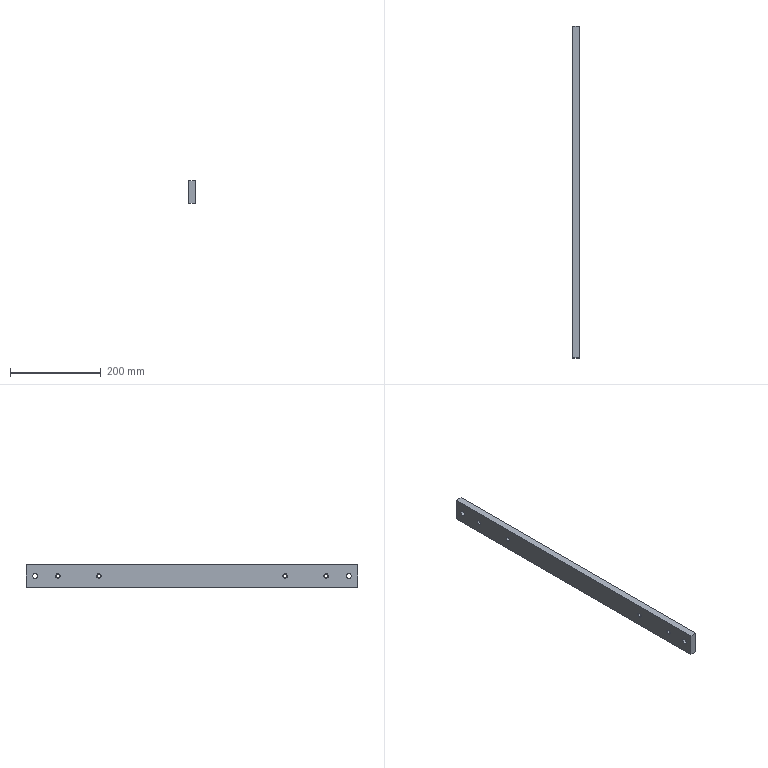Part | STEP file | Crossbeam | 1 solid | 20 faces | box 15 x 730 x 50 mm | volume 541334 mm3 | cone 8 | plane 6 | cylinder 6 | commonest cylinder face diameters 8.5 x4 10.7 x2